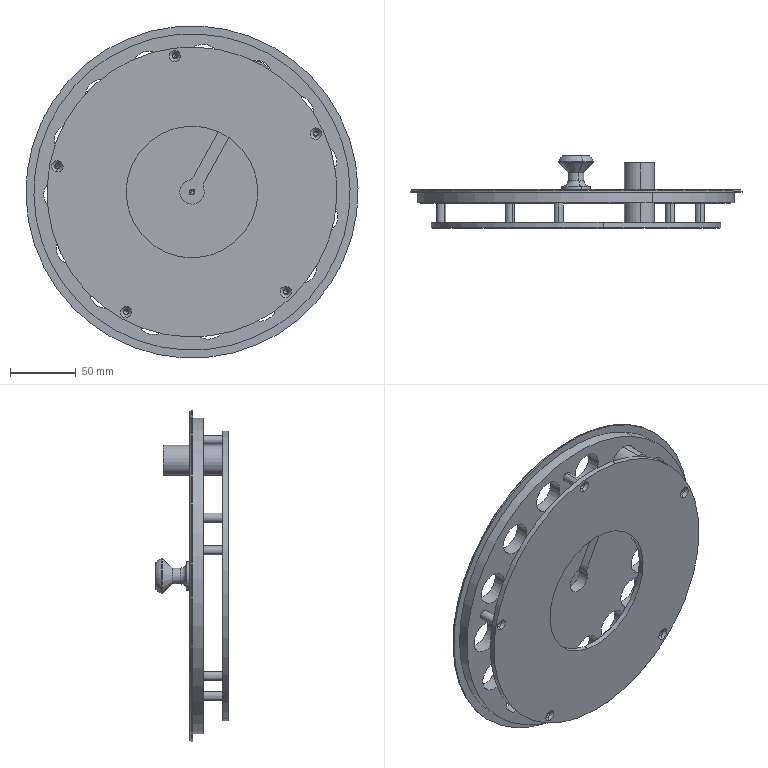Part | SolidWorks | 9 solids | 860 faces | box 252 x 54.8 x 252 mm | volume 440411 mm3 | plane 437 | spline 224 | cylinder 129 | cone 66 | torus 4 | commonest cylinder face diameters 25 x60 4.5 x22 3.3 x12 7 x10 10 x2 12 x2